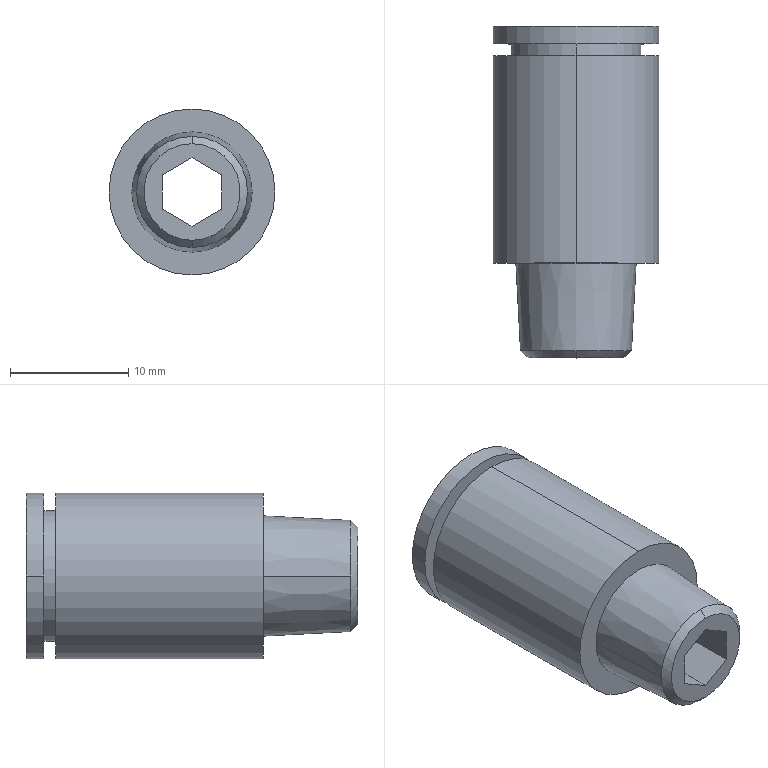Part | STEP file | 1 solid | 24 faces | box 14 x 28 x 14 mm | volume 2474 mm3 | plane 12 | cylinder 8 | cone 4 | commonest cylinder face diameters 14 x4 8 x2 11 x2